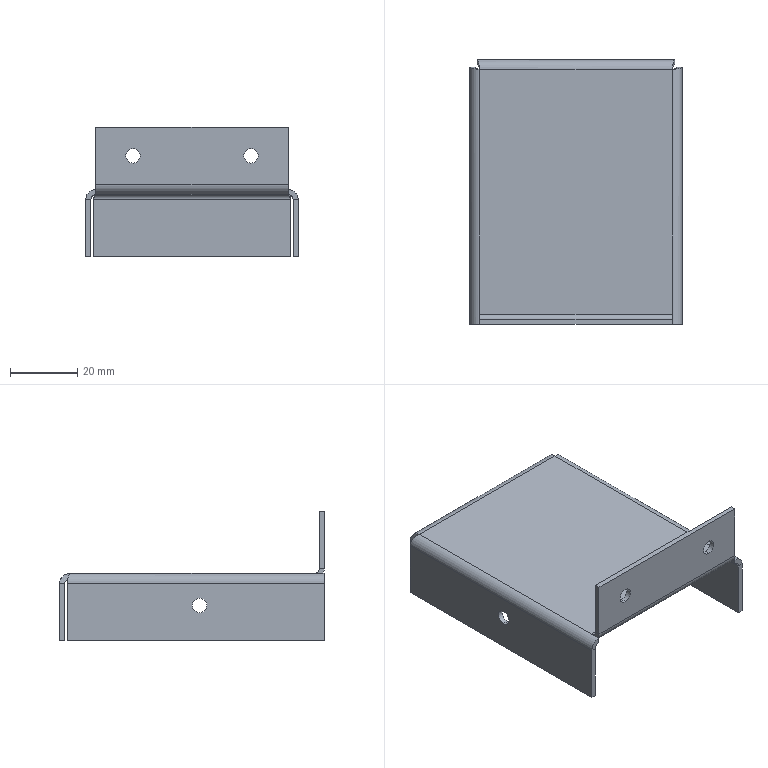Part | STEP file | Guard box plug SGN-3-07 | 1 solid | 48 faces | box 63 x 78.5 x 38.5 mm | volume 14363 mm3 | plane 28 | cylinder 16 | spline 4 | commonest cylinder face diameters 4.3 x8 3 x4 6 x4